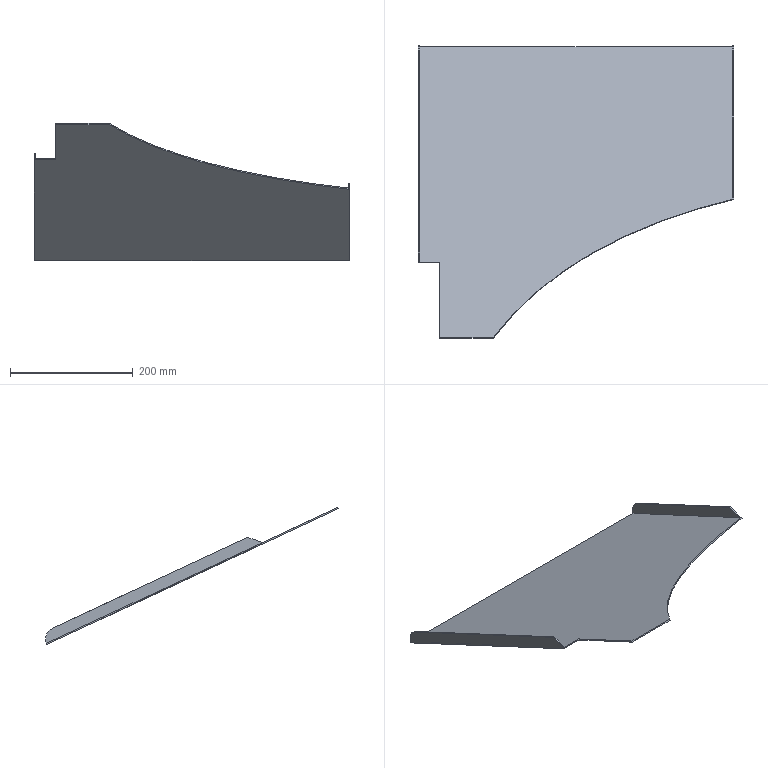Part | NX | features solid 2 | 1 solid | 17 faces | box 515 x 478.276 x 223.963 mm | volume 430449 mm3 | plane 14 | cylinder 2 | spline 1 | commonest cylinder face diameters 40 x2
STEP:
#1=CARTESIAN_POINT('',(-287.,720.,-282.15));
#2=VERTEX_POINT('',#1);
#3=CARTESIAN_POINT('',(-287.,720.,-279.943));
#4=VERTEX_POINT('',#3);
#5=CARTESIAN_POINT('',(-287.,720.,-430.));
#6=DIRECTION('',(0.,0.,1.));
#7=VECTOR('',#6,1000.);
#8=LINE('',#5,#7);
#9=EDGE_CURVE('',#2,#4,#8,.T.);
#10=ORIENTED_EDGE('',*,*,#9,.F.);
#11=CARTESIAN_POINT('',(-798.,720.,-282.15));
#12=VERTEX_POINT('',#11);
#13=CARTESIAN_POINT('',(188.564,720.,-282.15));
#14=DIRECTION('',(-1.,0.,0.));
#15=VECTOR('',#14,1000.);
#16=LINE('',#13,#15);
#17=EDGE_CURVE('',#2,#12,#16,.T.);
#18=ORIENTED_EDGE('',*,*,#17,.T.);
#19=CARTESIAN_POINT('',(-798.,720.,-279.943));
#20=VERTEX_POINT('',#19);
#21=CARTESIAN_POINT('',(-798.,720.,-430.));
#22=DIRECTION('',(0.,0.,-1.));
#23=VECTOR('',#22,1000.);
#24=LINE('',#21,#23);
#25=EDGE_CURVE('',#20,#12,#24,.T.);
#26=ORIENTED_EDGE('',*,*,#25,.F.);
#27=CARTESIAN_POINT('',(188.564,720.,-279.943));
#28=DIRECTION('',(-1.,0.,0.));
#29=VECTOR('',#28,1000.);
#30=LINE('',#27,#29);
#31=EDGE_CURVE('',#4,#20,#30,.T.);
#32=ORIENTED_EDGE('',*,*,#31,.F.);
#33=EDGE_LOOP('',(#10,#18,#26,#32));
#34=FACE_BOUND('',#33,.T.);
#35=CARTESIAN_POINT('',(188.564,720.,-430.));
#36=DIRECTION('',(0.,-1.,0.));
#37=DIRECTION('',(-1.,0.,0.));
#38=AXIS2_PLACEMENT_3D('',#35,#36,#37);
#39=PLANE('',#38);
#40=ADVANCED_FACE('',(#34),#39,.F.);
#41=CARTESIAN_POINT('',(-287.,472.974,-164.753));
#42=VERTEX_POINT('',#41);
#43=CARTESIAN_POINT('',(-285.,472.974,-164.753));
#44=VERTEX_POINT('',#43);
#45=CARTESIAN_POINT('',(-353.018,472.974,-164.753));
#46=DIRECTION('',(-1.,0.,0.));
#47=VECTOR('',#46,1000.);
#48=LINE('',#45,#47);
#49=EDGE_CURVE('',#42,#44,#48,.F.);
#50=ORIENTED_EDGE('',*,*,#49,.F.);
#51=CARTESIAN_POINT('',(-287.,417.055,-138.678));
#52=DIRECTION('',(0.,0.9063,-0.4226));
#53=VECTOR('',#52,1000.);
#54=LINE('',#51,#53);
#55=EDGE_CURVE('',#42,#4,#54,.T.);
#56=ORIENTED_EDGE('',*,*,#55,.T.);
#57=ORIENTED_EDGE('',*,*,#31,.T.);
#58=CARTESIAN_POINT('',(-798.,367.658,-115.644));
#59=VERTEX_POINT('',#58);
#60=CARTESIAN_POINT('',(-798.,417.055,-138.678));
#61=DIRECTION('',(0.,-0.9063,0.4226));
#62=VECTOR('',#61,1000.);
#63=LINE('',#60,#62);
#64=EDGE_CURVE('',#20,#59,#63,.T.);
#65=ORIENTED_EDGE('',*,*,#64,.T.);
#66=CARTESIAN_POINT('',(-765.,367.658,-115.644));
#67=VERTEX_POINT('',#66);
#68=CARTESIAN_POINT('',(-779.,367.658,-115.644));
#69=DIRECTION('',(-1.,0.,0.));
#70=VECTOR('',#69,1000.);
#71=LINE('',#68,#70);
#72=EDGE_CURVE('',#67,#59,#71,.T.);
#73=ORIENTED_EDGE('',*,*,#72,.F.);
#74=CARTESIAN_POINT('',(-765.,244.443,-58.187));
#75=VERTEX_POINT('',#74);
#76=CARTESIAN_POINT('',(-765.,272.567,-71.302));
#77=DIRECTION('',(0.,-0.9063,0.4226));
#78=VECTOR('',#77,1000.);
#79=LINE('',#76,#78);
#80=EDGE_CURVE('',#75,#67,#79,.F.);
#81=ORIENTED_EDGE('',*,*,#80,.F.);
#82=CARTESIAN_POINT('',(-677.72,244.443,-58.187));
#83=VERTEX_POINT('',#82);
#84=CARTESIAN_POINT('',(-353.018,244.443,-58.187));
#85=DIRECTION('',(1.,0.,0.));
#86=VECTOR('',#85,1000.);
#87=LINE('',#84,#86);
#88=EDGE_CURVE('',#75,#83,#87,.T.);
#89=ORIENTED_EDGE('',*,*,#88,.T.);
#90=CARTESIAN_POINT('',(-285.,471.162,-163.908));
#91=VERTEX_POINT('',#90);
#92=CARTESIAN_POINT('',(-677.72,244.443,-58.187));
#93=CARTESIAN_POINT('',(-672.167,251.77,-61.604));
#94=CARTESIAN_POINT('',(-663.423,262.605,-66.657));
#95=CARTESIAN_POINT('',(-650.978,276.698,-73.228));
#96=CARTESIAN_POINT('',(-641.165,287.179,-78.116));
#97=CARTESIAN_POINT('',(-631.216,297.219,-82.798));
#98=CARTESIAN_POINT('',(-620.962,307.004,-87.36));
#99=CARTESIAN_POINT('',(-612.158,314.946,-91.063));
#100=CARTESIAN_POINT('',(-604.955,321.177,-93.969));
#101=CARTESIAN_POINT('',(-600.401,325.008,-95.756));
#102=CARTESIAN_POINT('',(-596.688,328.067,-97.182));
#103=CARTESIAN_POINT('',(-593.065,331.011,-98.555));
#104=CARTESIAN_POINT('',(-586.789,336.01,-100.886));
#105=CARTESIAN_POINT('',(-573.857,345.914,-105.504));
#106=CARTESIAN_POINT('',(-558.47,356.808,-110.584));
#107=CARTESIAN_POINT('',(-542.419,367.323,-115.487));
#108=CARTESIAN_POINT('',(-530.057,375.012,-119.073));
#109=CARTESIAN_POINT('',(-517.377,382.503,-122.566));
#110=CARTESIAN_POINT('',(-506.516,388.595,-125.406));
#111=CARTESIAN_POINT('',(-498.82,392.748,-127.343));
#112=CARTESIAN_POINT('',(-494.304,395.136,-128.457));
#113=CARTESIAN_POINT('',(-490.241,397.26,-129.447));
#114=CARTESIAN_POINT('',(-484.961,399.97,-130.711));
#115=CARTESIAN_POINT('',(-476.523,404.197,-132.682));
#116=CARTESIAN_POINT('',(-465.791,409.379,-135.099));
#117=CARTESIAN_POINT('',(-448.313,417.413,-138.845));
#118=CARTESIAN_POINT('',(-430.339,425.076,-142.418));
#119=CARTESIAN_POINT('',(-411.886,432.361,-145.815));
#120=CARTESIAN_POINT('',(-400.134,436.764,-147.868));
#121=CARTESIAN_POINT('',(-390.645,440.181,-149.462));
#122=CARTESIAN_POINT('',(-383.373,442.729,-150.65));
#123=CARTESIAN_POINT('',(-376.401,445.108,-151.759));
#124=CARTESIAN_POINT('',(-367.079,448.209,-153.205));
#125=CARTESIAN_POINT('',(-357.741,451.192,-154.596));
#126=CARTESIAN_POINT('',(-348.382,454.06,-155.933));
#127=CARTESIAN_POINT('',(-341.353,456.153,-156.91));
#128=CARTESIAN_POINT('',(-335.488,457.849,-157.7));
#129=CARTESIAN_POINT('',(-330.79,459.178,-158.32));
#130=CARTESIAN_POINT('',(-327.855,459.995,-158.701));
#131=CARTESIAN_POINT('',(-325.793,460.562,-158.966));
#132=CARTESIAN_POINT('',(-324.625,460.882,-159.115));
#133=CARTESIAN_POINT('',(-323.869,461.088,-159.211));
#134=CARTESIAN_POINT('',(-323.323,461.236,-159.28));
#135=CARTESIAN_POINT('',(-322.949,461.338,-159.327));
#136=CARTESIAN_POINT('',(-322.199,461.541,-159.422));
#137=CARTESIAN_POINT('',(-320.706,461.943,-159.609));
#138=CARTESIAN_POINT('',(-318.393,462.561,-159.898));
#139=CARTESIAN_POINT('',(-314.394,463.619,-160.391));
#140=CARTESIAN_POINT('',(-308.795,465.082,-161.073));
#141=CARTESIAN_POINT('',(-302.405,466.73,-161.842));
#142=CARTESIAN_POINT('',(-297.517,467.981,-162.425));
#143=CARTESIAN_POINT('',(-294.603,468.725,-162.772));
#144=CARTESIAN_POINT('',(-292.74,469.199,-162.993));
#145=CARTESIAN_POINT('',(-291.2,469.59,-163.175));
#146=CARTESIAN_POINT('',(-290.27,469.826,-163.286));
#147=CARTESIAN_POINT('',(-289.417,470.043,-163.386));
#148=CARTESIAN_POINT('',(-288.93,470.166,-163.444));
#149=CARTESIAN_POINT('',(-287.978,470.408,-163.557));
#150=CARTESIAN_POINT('',(-286.649,470.744,-163.714));
#151=CARTESIAN_POINT('',(-285.552,471.022,-163.843));
#152=CARTESIAN_POINT('',(-285.,471.162,-163.908));
#153=B_SPLINE_CURVE_WITH_KNOTS('',3,(#92,#93,#94,#95,#96,#97,#98,#99,#100,#101,#102,#103,#104,#105,#106,#107,#108,#109,#110,#111,#112,#113,#114,#115,#116,#117,#118,#119,#120,#121,#122,#123,#124,#125,#126,#127,#128,#129,#130,#131,#132,#133,#134,#135,#136,#137,#138,#139,#140,#141,#142,#143,#144,#145,#146,#147,#148,#149,#150,#151,#152),.UNSPECIFIED.,.F.,.F.,(4,1,1,1,1,1,1,1,1,1,1,1,1,1,1,1,1,1,1,1,1,1,1,1,1,1,1,1,1,1,1,1,1,1,1,1,1,1,1,1,1,1,1,1,1,1,1,1,1,1,1,1,1,1,1,1,1,1,4),(0.,0.02989,0.04484,0.05979,0.07473,0.08968,0.1046,0.1121,0.1196,0.1233,0.127,0.1345,0.1495,0.1794,0.1943,0.2093,0.2242,0.2392,0.2466,0.2504,0.2541,0.2616,0.269,0.284,0.2989,0.3288,0.3438,0.3587,0.3662,0.3737,0.3811,0.3886,0.4036,0.411,0.4185,0.426,0.4297,0.4335,0.4353,0.4363,0.4372,0.4377,0.4381,0.4391,0.4409,0.4447,0.4484,0.4559,0.4634,0.4671,0.469,0.4708,0.4718,0.4727,0.4732,0.4736,0.4746,0.4764,0.4783),.UNSPECIFIED.);
#154=EDGE_CURVE('',#83,#91,#153,.T.);
#155=ORIENTED_EDGE('',*,*,#154,.T.);
#156=CARTESIAN_POINT('',(-285.,417.055,-138.678));
#157=DIRECTION('',(0.,0.9063,-0.4226));
#158=VECTOR('',#157,1000.);
#159=LINE('',#156,#158);
#160=EDGE_CURVE('',#91,#44,#159,.T.);
#161=ORIENTED_EDGE('',*,*,#160,.T.);
#162=EDGE_LOOP('',(#50,#56,#57,#65,#73,#81,#89,#155,#161));
#163=FACE_BOUND('',#162,.T.);
#164=CARTESIAN_POINT('',(-353.018,417.055,-138.678));
#165=DIRECTION('',(0.,0.4226,0.9063));
#166=DIRECTION('',(1.,0.,0.));
#167=AXIS2_PLACEMENT_3D('',#164,#165,#166);
#168=PLANE('',#167);
#169=ADVANCED_FACE('',(#163),#168,.T.);
#170=CARTESIAN_POINT('',(-285.,470.316,-165.721));
#171=VERTEX_POINT('',#170);
#172=CARTESIAN_POINT('',(-285.,471.162,-163.908));
#173=DIRECTION('',(0.,-0.4226,-0.9063));
#174=VECTOR('',#173,1000.);
#175=LINE('',#172,#174);
#176=EDGE_CURVE('',#91,#171,#175,.T.);
#177=ORIENTED_EDGE('',*,*,#176,.F.);
#178=ORIENTED_EDGE('',*,*,#154,.F.);
#179=CARTESIAN_POINT('',(-677.72,243.597,-60.));
#180=VERTEX_POINT('',#179);
#181=CARTESIAN_POINT('',(-677.72,243.597,-60.));
#182=CARTESIAN_POINT('',(-677.72,243.879,-59.396));
#183=CARTESIAN_POINT('',(-677.72,244.161,-58.792));
#184=CARTESIAN_POINT('',(-677.72,244.443,-58.187));
#185=B_SPLINE_CURVE_WITH_KNOTS('',3,(#181,#182,#183,#184),.UNSPECIFIED.,.F.,.F.,(4,4),(0.,1.),.UNSPECIFIED.);
#186=EDGE_CURVE('',#83,#180,#185,.F.);
#187=ORIENTED_EDGE('',*,*,#186,.T.);
#188=CARTESIAN_POINT('',(-677.72,243.597,-60.));
#189=CARTESIAN_POINT('',(-672.167,250.924,-63.417));
#190=CARTESIAN_POINT('',(-663.423,261.76,-68.469));
#191=CARTESIAN_POINT('',(-650.978,275.853,-75.041));
#192=CARTESIAN_POINT('',(-641.165,286.334,-79.928));
#193=CARTESIAN_POINT('',(-631.216,296.374,-84.61));
#194=CARTESIAN_POINT('',(-620.962,306.159,-89.173));
#195=CARTESIAN_POINT('',(-612.158,314.1,-92.876));
#196=CARTESIAN_POINT('',(-604.955,320.332,-95.782));
#197=CARTESIAN_POINT('',(-600.401,324.163,-97.568));
#198=CARTESIAN_POINT('',(-596.688,327.222,-98.995));
#199=CARTESIAN_POINT('',(-593.065,330.165,-100.367));
#200=CARTESIAN_POINT('',(-586.789,335.164,-102.698));
#201=CARTESIAN_POINT('',(-573.857,345.068,-107.317));
#202=CARTESIAN_POINT('',(-558.47,355.963,-112.397));
#203=CARTESIAN_POINT('',(-542.419,366.477,-117.3));
#204=CARTESIAN_POINT('',(-530.057,374.167,-120.886));
#205=CARTESIAN_POINT('',(-517.377,381.657,-124.378));
#206=CARTESIAN_POINT('',(-506.516,387.749,-127.219));
#207=CARTESIAN_POINT('',(-498.82,391.902,-129.156));
#208=CARTESIAN_POINT('',(-494.304,394.291,-130.27));
#209=CARTESIAN_POINT('',(-490.241,396.414,-131.26));
#210=CARTESIAN_POINT('',(-484.961,399.125,-132.524));
#211=CARTESIAN_POINT('',(-476.523,403.351,-134.494));
#212=CARTESIAN_POINT('',(-465.791,408.534,-136.911));
#213=CARTESIAN_POINT('',(-448.313,416.568,-140.657));
#214=CARTESIAN_POINT('',(-430.339,424.231,-144.231));
#215=CARTESIAN_POINT('',(-411.886,431.516,-147.628));
#216=CARTESIAN_POINT('',(-400.134,435.919,-149.681));
#217=CARTESIAN_POINT('',(-390.645,439.336,-151.274));
#218=CARTESIAN_POINT('',(-383.373,441.884,-152.463));
#219=CARTESIAN_POINT('',(-376.401,444.263,-153.572));
#220=CARTESIAN_POINT('',(-367.079,447.363,-155.018));
#221=CARTESIAN_POINT('',(-357.741,450.347,-156.409));
#222=CARTESIAN_POINT('',(-348.382,453.215,-157.746));
#223=CARTESIAN_POINT('',(-341.353,455.308,-158.722));
#224=CARTESIAN_POINT('',(-335.488,457.004,-159.513));
#225=CARTESIAN_POINT('',(-330.79,458.332,-160.133));
#226=CARTESIAN_POINT('',(-327.855,459.15,-160.514));
#227=CARTESIAN_POINT('',(-325.793,459.717,-160.778));
#228=CARTESIAN_POINT('',(-324.625,460.037,-160.927));
#229=CARTESIAN_POINT('',(-323.869,460.243,-161.023));
#230=CARTESIAN_POINT('',(-323.323,460.391,-161.093));
#231=CARTESIAN_POINT('',(-322.949,460.493,-161.14));
#232=CARTESIAN_POINT('',(-322.199,460.696,-161.235));
#233=CARTESIAN_POINT('',(-320.706,461.098,-161.422));
#234=CARTESIAN_POINT('',(-318.393,461.716,-161.71));
#235=CARTESIAN_POINT('',(-314.394,462.773,-162.203));
#236=CARTESIAN_POINT('',(-308.795,464.237,-162.886));
#237=CARTESIAN_POINT('',(-302.405,465.885,-163.654));
#238=CARTESIAN_POINT('',(-297.517,467.136,-164.238));
#239=CARTESIAN_POINT('',(-294.603,467.88,-164.584));
#240=CARTESIAN_POINT('',(-292.74,468.354,-164.806));
#241=CARTESIAN_POINT('',(-291.2,468.745,-164.988));
#242=CARTESIAN_POINT('',(-290.27,468.981,-165.098));
#243=CARTESIAN_POINT('',(-289.417,469.198,-165.199));
#244=CARTESIAN_POINT('',(-288.93,469.321,-165.257));
#245=CARTESIAN_POINT('',(-287.978,469.562,-165.369));
#246=CARTESIAN_POINT('',(-286.649,469.899,-165.526));
#247=CARTESIAN_POINT('',(-285.552,470.177,-165.656));
#248=CARTESIAN_POINT('',(-285.,470.316,-165.721));
#249=B_SPLINE_CURVE_WITH_KNOTS('',3,(#188,#189,#190,#191,#192,#193,#194,#195,#196,#197,#198,#199,#200,#201,#202,#203,#204,#205,#206,#207,#208,#209,#210,#211,#212,#213,#214,#215,#216,#217,#218,#219,#220,#221,#222,#223,#224,#225,#226,#227,#228,#229,#230,#231,#232,#233,#234,#235,#236,#237,#238,#239,#240,#241,#242,#243,#244,#245,#246,#247,#248),.UNSPECIFIED.,.F.,.F.,(4,1,1,1,1,1,1,1,1,1,1,1,1,1,1,1,1,1,1,1,1,1,1,1,1,1,1,1,1,1,1,1,1,1,1,1,1,1,1,1,1,1,1,1,1,1,1,1,1,1,1,1,1,1,1,1,1,1,4),(0.,0.02989,0.04484,0.05979,0.07473,0.08968,0.1046,0.1121,0.1196,0.1233,0.127,0.1345,0.1495,0.1794,0.1943,0.2093,0.2242,0.2392,0.2466,0.2504,0.2541,0.2616,0.269,0.284,0.2989,0.3288,0.3438,0.3587,0.3662,0.3737,0.3811,0.3886,0.4036,0.411,0.4185,0.426,0.4297,0.4335,0.4353,0.4363,0.4372,0.4377,0.4381,0.4391,0.4409,0.4447,0.4484,0.4559,0.4634,0.4671,0.469,0.4708,0.4718,0.4727,0.4732,0.4736,0.4746,0.4764,0.4783),.UNSPECIFIED.);
#250=EDGE_CURVE('',#180,#171,#249,.T.);
#251=ORIENTED_EDGE('',*,*,#250,.T.);
#252=EDGE_LOOP('',(#177,#178,#187,#251));
#253=FACE_BOUND('',#252,.T.);
#254=CARTESIAN_POINT('',(-677.72,244.443,-58.187));
#255=CARTESIAN_POINT('',(-677.72,243.597,-60.));
#256=CARTESIAN_POINT('',(-672.167,251.77,-61.604));
#257=CARTESIAN_POINT('',(-672.167,250.924,-63.417));
#258=CARTESIAN_POINT('',(-663.423,262.605,-66.657));
#259=CARTESIAN_POINT('',(-663.423,261.76,-68.469));
#260=CARTESIAN_POINT('',(-650.978,276.698,-73.228));
#261=CARTESIAN_POINT('',(-650.978,275.853,-75.041));
#262=CARTESIAN_POINT('',(-641.165,287.179,-78.116));
#263=CARTESIAN_POINT('',(-641.165,286.334,-79.928));
#264=CARTESIAN_POINT('',(-631.216,297.219,-82.798));
#265=CARTESIAN_POINT('',(-631.216,296.374,-84.61));
#266=CARTESIAN_POINT('',(-620.962,307.004,-87.36));
#267=CARTESIAN_POINT('',(-620.962,306.159,-89.173));
#268=CARTESIAN_POINT('',(-612.158,314.946,-91.063));
#269=CARTESIAN_POINT('',(-612.158,314.1,-92.876));
#270=CARTESIAN_POINT('',(-604.955,321.177,-93.969));
#271=CARTESIAN_POINT('',(-604.955,320.332,-95.782));
#272=CARTESIAN_POINT('',(-600.401,325.008,-95.756));
#273=CARTESIAN_POINT('',(-600.401,324.163,-97.568));
#274=CARTESIAN_POINT('',(-596.688,328.067,-97.182));
#275=CARTESIAN_POINT('',(-596.688,327.222,-98.995));
#276=CARTESIAN_POINT('',(-593.065,331.011,-98.555));
#277=CARTESIAN_POINT('',(-593.065,330.165,-100.367));
#278=CARTESIAN_POINT('',(-586.789,336.01,-100.886));
#279=CARTESIAN_POINT('',(-586.789,335.164,-102.698));
#280=CARTESIAN_POINT('',(-573.857,345.914,-105.504));
#281=CARTESIAN_POINT('',(-573.857,345.068,-107.317));
#282=CARTESIAN_POINT('',(-558.47,356.808,-110.584));
#283=CARTESIAN_POINT('',(-558.47,355.963,-112.397));
#284=CARTESIAN_POINT('',(-542.419,367.323,-115.487));
#285=CARTESIAN_POINT('',(-542.419,366.477,-117.3));
#286=CARTESIAN_POINT('',(-530.057,375.012,-119.073));
#287=CARTESIAN_POINT('',(-530.057,374.167,-120.886));
#288=CARTESIAN_POINT('',(-517.377,382.503,-122.566));
#289=CARTESIAN_POINT('',(-517.377,381.657,-124.378));
#290=CARTESIAN_POINT('',(-506.516,388.595,-125.406));
#291=CARTESIAN_POINT('',(-506.516,387.749,-127.219));
#292=CARTESIAN_POINT('',(-498.82,392.748,-127.343));
#293=CARTESIAN_POINT('',(-498.82,391.902,-129.156));
#294=CARTESIAN_POINT('',(-494.304,395.136,-128.457));
#295=CARTESIAN_POINT('',(-494.304,394.291,-130.27));
#296=CARTESIAN_POINT('',(-490.241,397.26,-129.447));
#297=CARTESIAN_POINT('',(-490.241,396.414,-131.26));
#298=CARTESIAN_POINT('',(-484.961,399.97,-130.711));
#299=CARTESIAN_POINT('',(-484.961,399.125,-132.524));
#300=CARTESIAN_POINT('',(-476.523,404.197,-132.682));
#301=CARTESIAN_POINT('',(-476.523,403.351,-134.494));
#302=CARTESIAN_POINT('',(-465.791,409.379,-135.099));
#303=CARTESIAN_POINT('',(-465.791,408.534,-136.911));
#304=CARTESIAN_POINT('',(-448.313,417.413,-138.845));
#305=CARTESIAN_POINT('',(-448.313,416.568,-140.657));
#306=CARTESIAN_POINT('',(-430.339,425.076,-142.418));
#307=CARTESIAN_POINT('',(-430.339,424.231,-144.231));
#308=CARTESIAN_POINT('',(-411.886,432.361,-145.815));
#309=CARTESIAN_POINT('',(-411.886,431.516,-147.628));
#310=CARTESIAN_POINT('',(-400.134,436.764,-147.868));
#311=CARTESIAN_POINT('',(-400.134,435.919,-149.681));
#312=CARTESIAN_POINT('',(-390.645,440.181,-149.462));
#313=CARTESIAN_POINT('',(-390.645,439.336,-151.274));
#314=CARTESIAN_POINT('',(-383.373,442.729,-150.65));
#315=CARTESIAN_POINT('',(-383.373,441.884,-152.463));
#316=CARTESIAN_POINT('',(-376.401,445.108,-151.759));
#317=CARTESIAN_POINT('',(-376.401,444.263,-153.572));
#318=CARTESIAN_POINT('',(-367.079,448.209,-153.205));
#319=CARTESIAN_POINT('',(-367.079,447.363,-155.018));
#320=CARTESIAN_POINT('',(-357.741,451.192,-154.596));
#321=CARTESIAN_POINT('',(-357.741,450.347,-156.409));
#322=CARTESIAN_POINT('',(-348.382,454.06,-155.933));
#323=CARTESIAN_POINT('',(-348.382,453.215,-157.746));
#324=CARTESIAN_POINT('',(-341.353,456.153,-156.91));
#325=CARTESIAN_POINT('',(-341.353,455.308,-158.722));
#326=CARTESIAN_POINT('',(-335.488,457.849,-157.7));
#327=CARTESIAN_POINT('',(-335.488,457.004,-159.513));
#328=CARTESIAN_POINT('',(-330.79,459.178,-158.32));
#329=CARTESIAN_POINT('',(-330.79,458.332,-160.133));
#330=CARTESIAN_POINT('',(-327.855,459.995,-158.701));
#331=CARTESIAN_POINT('',(-327.855,459.15,-160.514));
#332=CARTESIAN_POINT('',(-325.793,460.562,-158.966));
#333=CARTESIAN_POINT('',(-325.793,459.717,-160.778));
#334=CARTESIAN_POINT('',(-324.625,460.882,-159.115));
#335=CARTESIAN_POINT('',(-324.625,460.037,-160.927));
#336=CARTESIAN_POINT('',(-323.869,461.088,-159.211));
#337=CARTESIAN_POINT('',(-323.869,460.243,-161.023));
#338=CARTESIAN_POINT('',(-323.323,461.236,-159.28));
#339=CARTESIAN_POINT('',(-323.323,460.391,-161.093));
#340=CARTESIAN_POINT('',(-322.949,461.338,-159.327));
#341=CARTESIAN_POINT('',(-322.949,460.493,-161.14));
#342=CARTESIAN_POINT('',(-322.199,461.541,-159.422));
#343=CARTESIAN_POINT('',(-322.199,460.696,-161.235));
#344=CARTESIAN_POINT('',(-320.706,461.943,-159.609));
#345=CARTESIAN_POINT('',(-320.706,461.098,-161.422));
#346=CARTESIAN_POINT('',(-318.393,462.561,-159.898));
#347=CARTESIAN_POINT('',(-318.393,461.716,-161.71));
#348=CARTESIAN_POINT('',(-314.394,463.619,-160.391));
#349=CARTESIAN_POINT('',(-314.394,462.773,-162.203));
#350=CARTESIAN_POINT('',(-308.795,465.082,-161.073));
#351=CARTESIAN_POINT('',(-308.795,464.237,-162.886));
#352=CARTESIAN_POINT('',(-302.405,466.73,-161.842));
#353=CARTESIAN_POINT('',(-302.405,465.885,-163.654));
#354=CARTESIAN_POINT('',(-297.517,467.981,-162.425));
#355=CARTESIAN_POINT('',(-297.517,467.136,-164.238));
#356=CARTESIAN_POINT('',(-294.603,468.725,-162.772));
#357=CARTESIAN_POINT('',(-294.603,467.88,-164.584));
#358=CARTESIAN_POINT('',(-292.74,469.199,-162.993));
#359=CARTESIAN_POINT('',(-292.74,468.354,-164.806));
#360=CARTESIAN_POINT('',(-291.2,469.59,-163.175));
#361=CARTESIAN_POINT('',(-291.2,468.745,-164.988));
#362=CARTESIAN_POINT('',(-290.27,469.826,-163.286));
#363=CARTESIAN_POINT('',(-290.27,468.981,-165.098));
#364=CARTESIAN_POINT('',(-289.417,470.043,-163.386));
#365=CARTESIAN_POINT('',(-289.417,469.198,-165.199));
#366=CARTESIAN_POINT('',(-288.93,470.166,-163.444));
#367=CARTESIAN_POINT('',(-288.93,469.321,-165.257));
#368=CARTESIAN_POINT('',(-287.978,470.408,-163.557));
#369=CARTESIAN_POINT('',(-287.978,469.562,-165.369));
#370=CARTESIAN_POINT('',(-286.649,470.744,-163.714));
#371=CARTESIAN_POINT('',(-286.649,469.899,-165.526));
#372=CARTESIAN_POINT('',(-285.552,471.022,-163.843));
#373=CARTESIAN_POINT('',(-285.552,470.177,-165.656));
#374=CARTESIAN_POINT('',(-285.,471.162,-163.908));
#375=CARTESIAN_POINT('',(-285.,470.316,-165.721));
#376=B_SPLINE_SURFACE_WITH_KNOTS('',3,1,((#254,#255),(#256,#257),(#258,#259),(#260,#261),(#262,#263),(#264,#265),(#266,#267),(#268,#269),(#270,#271),(#272,#273),(#274,#275),(#276,#277),(#278,#279),(#280,#281),(#282,#283),(#284,#285),(#286,#287),(#288,#289),(#290,#291),(#292,#293),(#294,#295),(#296,#297),(#298,#299),(#300,#301),(#302,#303),(#304,#305),(#306,#307),(#308,#309),(#310,#311),(#312,#313),(#314,#315),(#316,#317),(#318,#319),(#320,#321),(#322,#323),(#324,#325),(#326,#327),(#328,#329),(#330,#331),(#332,#333),(#334,#335),(#336,#337),(#338,#339),(#340,#341),(#342,#343),(#344,#345),(#346,#347),(#348,#349),(#350,#351),(#352,#353),(#354,#355),(#356,#357),(#358,#359),(#360,#361),(#362,#363),(#364,#365),(#366,#367),(#368,#369),(#370,#371),(#372,#373),(#374,#375)),.SURF_OF_LINEAR_EXTRUSION.,.F.,.F.,.F.,(4,1,1,1,1,1,1,1,1,1,1,1,1,1,1,1,1,1,1,1,1,1,1,1,1,1,1,1,1,1,1,1,1,1,1,1,1,1,1,1,1,1,1,1,1,1,1,1,1,1,1,1,1,1,1,1,1,1,4),(2,2),(0.,0.02989,0.04484,0.05979,0.07473,0.08968,0.1046,0.1121,0.1196,0.1233,0.127,0.1345,0.1495,0.1794,0.1943,0.2093,0.2242,0.2392,0.2466,0.2504,0.2541,0.2616,0.269,0.284,0.2989,0.3288,0.3438,0.3587,0.3662,0.3737,0.3811,0.3886,0.4036,0.411,0.4185,0.426,0.4297,0.4335,0.4353,0.4363,0.4372,0.4377,0.4381,0.4391,0.4409,0.4447,0.4484,0.4559,0.4634,0.4671,0.469,0.4708,0.4718,0.4727,0.4732,0.4736,0.4746,0.4764,0.4783),(0.,1.),.UNSPECIFIED.);
#377=ADVANCED_FACE('',(#253),#376,.F.);
#378=ORIENTED_EDGE('',*,*,#17,.F.);
#379=CARTESIAN_POINT('',(-285.,720.,-282.15));
#380=VERTEX_POINT('',#379);
#381=CARTESIAN_POINT('',(188.564,720.,-282.15));
#382=DIRECTION('',(-1.,0.,0.));
#383=VECTOR('',#382,1000.);
#384=LINE('',#381,#383);
#385=EDGE_CURVE('',#380,#2,#384,.T.);
#386=ORIENTED_EDGE('',*,*,#385,.F.);
#387=CARTESIAN_POINT('',(-285.,416.21,-140.491));
#388=DIRECTION('',(0.,0.9063,-0.4226));
#389=VECTOR('',#388,1000.);
#390=LINE('',#387,#389);
#391=EDGE_CURVE('',#171,#380,#390,.T.);
#392=ORIENTED_EDGE('',*,*,#391,.F.);
#393=ORIENTED_EDGE('',*,*,#250,.F.);
#394=CARTESIAN_POINT('',(-765.,243.597,-60.));
#395=VERTEX_POINT('',#394);
#396=CARTESIAN_POINT('',(-353.018,243.597,-60.));
#397=DIRECTION('',(1.,0.,0.));
#398=VECTOR('',#397,1000.);
#399=LINE('',#396,#398);
#400=EDGE_CURVE('',#395,#180,#399,.T.);
#401=ORIENTED_EDGE('',*,*,#400,.F.);
#402=CARTESIAN_POINT('',(-765.,366.813,-117.456));
#403=VERTEX_POINT('',#402);
#404=CARTESIAN_POINT('',(-765.,271.722,-73.114));
#405=DIRECTION('',(0.,-0.9063,0.4226));
#406=VECTOR('',#405,1000.);
#407=LINE('',#404,#406);
#408=EDGE_CURVE('',#395,#403,#407,.F.);
#409=ORIENTED_EDGE('',*,*,#408,.T.);
#410=CARTESIAN_POINT('',(-800.,366.813,-117.456));
#411=VERTEX_POINT('',#410);
#412=CARTESIAN_POINT('',(-779.,366.813,-117.456));
#413=DIRECTION('',(-1.,0.,0.));
#414=VECTOR('',#413,1000.);
#415=LINE('',#412,#414);
#416=EDGE_CURVE('',#403,#411,#415,.T.);
#417=ORIENTED_EDGE('',*,*,#416,.T.);
#418=CARTESIAN_POINT('',(-800.,720.,-282.15));
#419=VERTEX_POINT('',#418);
#420=CARTESIAN_POINT('',(-800.,559.597,-207.353));
#421=DIRECTION('',(0.,-0.9063,0.4226));
#422=VECTOR('',#421,1000.);
#423=LINE('',#420,#422);
#424=EDGE_CURVE('',#419,#411,#423,.T.);
#425=ORIENTED_EDGE('',*,*,#424,.F.);
#426=CARTESIAN_POINT('',(-800.,720.,-282.15));
#427=DIRECTION('',(1.,0.,0.));
#428=VECTOR('',#427,1000.);
#429=LINE('',#426,#428);
#430=EDGE_CURVE('',#419,#12,#429,.T.);
#431=ORIENTED_EDGE('',*,*,#430,.T.);
#432=EDGE_LOOP('',(#378,#386,#392,#393,#401,#409,#417,#425,#431));
#433=FACE_BOUND('',#432,.T.);
#434=CARTESIAN_POINT('',(-353.018,416.21,-140.491));
#435=DIRECTION('',(0.,0.4226,0.9063));
#436=DIRECTION('',(1.,0.,0.));
#437=AXIS2_PLACEMENT_3D('',#434,#435,#436);
#438=PLANE('',#437);
#439=ADVANCED_FACE('',(#433),#438,.F.);
#440=ORIENTED_EDGE('',*,*,#72,.T.);
#441=CARTESIAN_POINT('',(-800.,367.658,-115.644));
#442=VERTEX_POINT('',#441);
#443=CARTESIAN_POINT('',(-779.,367.658,-115.644));
#444=DIRECTION('',(-1.,0.,0.));
#445=VECTOR('',#444,1000.);
#446=LINE('',#443,#445);
#447=EDGE_CURVE('',#59,#442,#446,.T.);
#448=ORIENTED_EDGE('',*,*,#447,.T.);
#449=CARTESIAN_POINT('',(-800.,367.658,-115.644));
#450=DIRECTION('',(0.,-0.4226,-0.9063));
#451=VECTOR('',#450,1000.);
#452=LINE('',#449,#451);
#453=EDGE_CURVE('',#442,#411,#452,.T.);
#454=ORIENTED_EDGE('',*,*,#453,.T.);
#455=ORIENTED_EDGE('',*,*,#416,.F.);
#456=CARTESIAN_POINT('',(-765.,367.658,-115.644));
#457=DIRECTION('',(0.,-0.4226,-0.9063));
#458=VECTOR('',#457,1000.);
#459=LINE('',#456,#458);
#460=EDGE_CURVE('',#67,#403,#459,.T.);
#461=ORIENTED_EDGE('',*,*,#460,.F.);
#462=EDGE_LOOP('',(#440,#448,#454,#455,#461));
#463=FACE_BOUND('',#462,.T.);
#464=CARTESIAN_POINT('',(-779.,367.658,-115.644));
#465=DIRECTION('',(0.,-0.9063,0.4226));
#466=DIRECTION('',(0.,-0.4226,-0.9063));
#467=AXIS2_PLACEMENT_3D('',#464,#465,#466);
#468=PLANE('',#467);
#469=ADVANCED_FACE('',(#463),#468,.T.);
#470=ORIENTED_EDGE('',*,*,#408,.F.);
#471=CARTESIAN_POINT('',(-765.,244.443,-58.187));
#472=DIRECTION('',(0.,0.4226,0.9063));
#473=VECTOR('',#472,1000.);
#474=LINE('',#471,#473);
#475=EDGE_CURVE('',#395,#75,#474,.T.);
#476=ORIENTED_EDGE('',*,*,#475,.T.);
#477=ORIENTED_EDGE('',*,*,#80,.T.);
#478=ORIENTED_EDGE('',*,*,#460,.T.);
#479=EDGE_LOOP('',(#470,#476,#477,#478));
#480=FACE_BOUND('',#479,.T.);
#481=CARTESIAN_POINT('',(-765.,272.567,-71.302));
#482=DIRECTION('',(-1.,0.,0.));
#483=DIRECTION('',(0.,0.,1.));
#484=AXIS2_PLACEMENT_3D('',#481,#482,#483);
#485=PLANE('',#484);
#486=ADVANCED_FACE('',(#480),#485,.T.);
#487=ORIENTED_EDGE('',*,*,#475,.F.);
#488=ORIENTED_EDGE('',*,*,#400,.T.);
#489=ORIENTED_EDGE('',*,*,#186,.F.);
#490=ORIENTED_EDGE('',*,*,#88,.F.);
#491=EDGE_LOOP('',(#487,#488,#489,#490));
#492=FACE_BOUND('',#491,.T.);
#493=CARTESIAN_POINT('',(-353.018,244.443,-58.187));
#494=DIRECTION('',(0.,0.9063,-0.4226));
#495=DIRECTION('',(0.,0.4226,0.9063));
#496=AXIS2_PLACEMENT_3D('',#493,#494,#495);
#497=PLANE('',#496);
#498=ADVANCED_FACE('',(#492),#497,.F.);
#499=ORIENTED_EDGE('',*,*,#453,.F.);
#500=CARTESIAN_POINT('',(-800.,391.579,-106.937));
#501=VERTEX_POINT('',#500);
#502=CARTESIAN_POINT('',(-800.,367.658,-115.644));
#503=DIRECTION('',(0.,0.9397,0.342));
#504=VECTOR('',#503,1000.);
#505=LINE('',#502,#504);
#506=EDGE_CURVE('',#442,#501,#505,.T.);
#507=ORIENTED_EDGE('',*,*,#506,.T.);
#508=CARTESIAN_POINT('',(-800.,710.326,-255.572));
#509=VERTEX_POINT('',#508);
#510=CARTESIAN_POINT('',(-800.,728.452,-264.024));
#511=DIRECTION('',(0.,-0.9063,0.4226));
#512=VECTOR('',#511,1000.);
#513=LINE('',#510,#512);
#514=EDGE_CURVE('',#509,#501,#513,.T.);
#515=ORIENTED_EDGE('',*,*,#514,.F.);
#516=CARTESIAN_POINT('',(-800.,701.874,-273.698));
#517=DIRECTION('',(-1.,0.,0.));
#518=DIRECTION('',(0.,0.,1.));
#519=AXIS2_PLACEMENT_3D('',#516,#517,#518);
#520=CIRCLE('',#519,20.);
#521=EDGE_CURVE('',#509,#419,#520,.T.);
#522=ORIENTED_EDGE('',*,*,#521,.T.);
#523=ORIENTED_EDGE('',*,*,#424,.T.);
#524=EDGE_LOOP('',(#499,#507,#515,#522,#523));
#525=FACE_BOUND('',#524,.T.);
#526=CARTESIAN_POINT('',(-800.,560.442,-205.54));
#527=DIRECTION('',(1.,0.,0.));
#528=DIRECTION('',(0.,0.,-1.));
#529=AXIS2_PLACEMENT_3D('',#526,#527,#528);
#530=PLANE('',#529);
#531=ADVANCED_FACE('',(#525),#530,.F.);
#532=CARTESIAN_POINT('',(-798.,710.326,-255.572));
#533=VERTEX_POINT('',#532);
#534=CARTESIAN_POINT('',(-798.,391.579,-106.937));
#535=VERTEX_POINT('',#534);
#536=CARTESIAN_POINT('',(-798.,728.452,-264.024));
#537=DIRECTION('',(0.,-0.9063,0.4226));
#538=VECTOR('',#537,1000.);
#539=LINE('',#536,#538);
#540=EDGE_CURVE('',#533,#535,#539,.T.);
#541=ORIENTED_EDGE('',*,*,#540,.T.);
#542=CARTESIAN_POINT('',(-798.,367.658,-115.644));
#543=DIRECTION('',(0.,-0.9397,-0.342));
#544=VECTOR('',#543,1000.);
#545=LINE('',#542,#544);
#546=EDGE_CURVE('',#535,#59,#545,.T.);
#547=ORIENTED_EDGE('',*,*,#546,.T.);
#548=ORIENTED_EDGE('',*,*,#64,.F.);
#549=ORIENTED_EDGE('',*,*,#25,.T.);
#550=CARTESIAN_POINT('',(-798.,701.874,-273.698));
#551=DIRECTION('',(-1.,0.,0.));
#552=DIRECTION('',(0.,0.,1.));
#553=AXIS2_PLACEMENT_3D('',#550,#551,#552);
#554=CIRCLE('',#553,20.);
#555=EDGE_CURVE('',#12,#533,#554,.F.);
#556=ORIENTED_EDGE('',*,*,#555,.T.);
#557=EDGE_LOOP('',(#541,#547,#548,#549,#556));
#558=FACE_BOUND('',#557,.T.);
#559=CARTESIAN_POINT('',(-798.,720.,-282.15));
#560=DIRECTION('',(-1.,0.,0.));
#561=DIRECTION('',(0.,0.,1.));
#562=AXIS2_PLACEMENT_3D('',#559,#560,#561);
#563=PLANE('',#562);
#564=ADVANCED_FACE('',(#558),#563,.F.);
#565=ORIENTED_EDGE('',*,*,#514,.T.);
#566=CARTESIAN_POINT('',(-800.,391.579,-106.937));
#567=DIRECTION('',(-1.,0.,0.));
#568=VECTOR('',#567,1000.);
#569=LINE('',#566,#568);
#570=EDGE_CURVE('',#501,#535,#569,.F.);
#571=ORIENTED_EDGE('',*,*,#570,.T.);
#572=ORIENTED_EDGE('',*,*,#540,.F.);
#573=CARTESIAN_POINT('',(-800.,710.326,-255.572));
#574=DIRECTION('',(-1.,0.,0.));
#575=VECTOR('',#574,1000.);
#576=LINE('',#573,#575);
#577=EDGE_CURVE('',#533,#509,#576,.T.);
#578=ORIENTED_EDGE('',*,*,#577,.T.);
#579=EDGE_LOOP('',(#565,#571,#572,#578));
#580=FACE_BOUND('',#579,.T.);
#581=CARTESIAN_POINT('',(-800.,728.452,-264.024));
#582=DIRECTION('',(0.,-0.4226,-0.9063));
#583=DIRECTION('',(0.,-0.9063,0.4226));
#584=AXIS2_PLACEMENT_3D('',#581,#582,#583);
#585=PLANE('',#584);
#586=ADVANCED_FACE('',(#580),#585,.F.);
#587=ORIENTED_EDGE('',*,*,#521,.F.);
#588=ORIENTED_EDGE('',*,*,#577,.F.);
#589=ORIENTED_EDGE('',*,*,#555,.F.);
#590=ORIENTED_EDGE('',*,*,#430,.F.);
#591=EDGE_LOOP('',(#587,#588,#589,#590));
#592=FACE_BOUND('',#591,.T.);
#593=CARTESIAN_POINT('',(-800.,701.874,-273.698));
#594=DIRECTION('',(1.,0.,0.));
#595=DIRECTION('',(0.,0.,-1.));
#596=AXIS2_PLACEMENT_3D('',#593,#594,#595);
#597=CYLINDRICAL_SURFACE('',#596,20.);
#598=ADVANCED_FACE('',(#592),#597,.T.);
#599=ORIENTED_EDGE('',*,*,#176,.T.);
#600=ORIENTED_EDGE('',*,*,#391,.T.);
#601=CARTESIAN_POINT('',(-285.,710.326,-255.572));
#602=VERTEX_POINT('',#601);
#603=CARTESIAN_POINT('',(-285.,701.874,-273.698));
#604=DIRECTION('',(1.,0.,0.));
#605=DIRECTION('',(0.,0.,-1.));
#606=AXIS2_PLACEMENT_3D('',#603,#604,#605);
#607=CIRCLE('',#606,20.);
#608=EDGE_CURVE('',#380,#602,#607,.T.);
#609=ORIENTED_EDGE('',*,*,#608,.T.);
#610=CARTESIAN_POINT('',(-285.,496.895,-156.047));
#611=VERTEX_POINT('',#610);
#612=CARTESIAN_POINT('',(-285.,478.769,-147.595));
#613=DIRECTION('',(0.,0.9063,-0.4226));
#614=VECTOR('',#613,1000.);
#615=LINE('',#612,#614);
#616=EDGE_CURVE('',#611,#602,#615,.T.);
#617=ORIENTED_EDGE('',*,*,#616,.F.);
#618=CARTESIAN_POINT('',(-285.,470.316,-165.721));
#619=DIRECTION('',(0.,0.9397,0.342));
#620=VECTOR('',#619,1000.);
#621=LINE('',#618,#620);
#622=EDGE_CURVE('',#611,#44,#621,.F.);
#623=ORIENTED_EDGE('',*,*,#622,.T.);
#624=ORIENTED_EDGE('',*,*,#160,.F.);
#625=EDGE_LOOP('',(#599,#600,#609,#617,#623,#624));
#626=FACE_BOUND('',#625,.T.);
#627=CARTESIAN_POINT('',(-285.,610.,-55.));
#628=DIRECTION('',(1.,0.,0.));
#629=DIRECTION('',(0.,0.,-1.));
#630=AXIS2_PLACEMENT_3D('',#627,#628,#629);
#631=PLANE('',#630);
#632=ADVANCED_FACE('',(#626),#631,.T.);
#633=CARTESIAN_POINT('',(-287.,710.326,-255.572));
#634=VERTEX_POINT('',#633);
#635=CARTESIAN_POINT('',(-287.,701.874,-273.698));
#636=DIRECTION('',(1.,0.,0.));
#637=DIRECTION('',(0.,0.,-1.));
#638=AXIS2_PLACEMENT_3D('',#635,#636,#637);
#639=CIRCLE('',#638,20.);
#640=EDGE_CURVE('',#634,#2,#639,.F.);
#641=ORIENTED_EDGE('',*,*,#640,.T.);
#642=ORIENTED_EDGE('',*,*,#9,.T.);
#643=ORIENTED_EDGE('',*,*,#55,.F.);
#644=CARTESIAN_POINT('',(-287.,496.895,-156.047));
#645=VERTEX_POINT('',#644);
#646=CARTESIAN_POINT('',(-287.,470.316,-165.721));
#647=DIRECTION('',(0.,-0.9397,-0.342));
#648=VECTOR('',#647,1000.);
#649=LINE('',#646,#648);
#650=EDGE_CURVE('',#42,#645,#649,.F.);
#651=ORIENTED_EDGE('',*,*,#650,.T.);
#652=CARTESIAN_POINT('',(-287.,478.769,-147.595));
#653=DIRECTION('',(0.,0.9063,-0.4226));
#654=VECTOR('',#653,1000.);
#655=LINE('',#652,#654);
#656=EDGE_CURVE('',#645,#634,#655,.T.);
#657=ORIENTED_EDGE('',*,*,#656,.T.);
#658=EDGE_LOOP('',(#641,#642,#643,#651,#657));
#659=FACE_BOUND('',#658,.T.);
#660=CARTESIAN_POINT('',(-287.,470.316,-165.721));
#661=DIRECTION('',(1.,0.,0.));
#662=DIRECTION('',(0.,0.,-1.));
#663=AXIS2_PLACEMENT_3D('',#660,#661,#662);
#664=PLANE('',#663);
#665=ADVANCED_FACE('',(#659),#664,.F.);
#666=ORIENTED_EDGE('',*,*,#616,.T.);
#667=CARTESIAN_POINT('',(-285.,710.326,-255.572));
#668=DIRECTION('',(1.,0.,0.));
#669=VECTOR('',#668,1000.);
#670=LINE('',#667,#669);
#671=EDGE_CURVE('',#602,#634,#670,.F.);
#672=ORIENTED_EDGE('',*,*,#671,.T.);
#673=ORIENTED_EDGE('',*,*,#656,.F.);
#674=CARTESIAN_POINT('',(-285.,496.895,-156.047));
#675=DIRECTION('',(1.,0.,0.));
#676=VECTOR('',#675,1000.);
#677=LINE('',#674,#676);
#678=EDGE_CURVE('',#645,#611,#677,.T.);
#679=ORIENTED_EDGE('',*,*,#678,.T.);
#680=EDGE_LOOP('',(#666,#672,#673,#679));
#681=FACE_BOUND('',#680,.T.);
#682=CARTESIAN_POINT('',(-285.,478.769,-147.595));
#683=DIRECTION('',(0.,-0.4226,-0.9063));
#684=DIRECTION('',(0.,0.9063,-0.4226));
#685=AXIS2_PLACEMENT_3D('',#682,#683,#684);
#686=PLANE('',#685);
#687=ADVANCED_FACE('',(#681),#686,.F.);
#688=ORIENTED_EDGE('',*,*,#650,.F.);
#689=ORIENTED_EDGE('',*,*,#49,.T.);
#690=ORIENTED_EDGE('',*,*,#622,.F.);
#691=ORIENTED_EDGE('',*,*,#678,.F.);
#692=EDGE_LOOP('',(#688,#689,#690,#691));
#693=FACE_BOUND('',#692,.T.);
#694=CARTESIAN_POINT('',(-285.,470.316,-165.721));
#695=DIRECTION('',(0.,0.342,-0.9397));
#696=DIRECTION('',(0.,0.9397,0.342));
#697=AXIS2_PLACEMENT_3D('',#694,#695,#696);
#698=PLANE('',#697);
#699=ADVANCED_FACE('',(#693),#698,.F.);
#700=ORIENTED_EDGE('',*,*,#608,.F.);
#701=ORIENTED_EDGE('',*,*,#385,.T.);
#702=ORIENTED_EDGE('',*,*,#640,.F.);
#703=ORIENTED_EDGE('',*,*,#671,.F.);
#704=EDGE_LOOP('',(#700,#701,#702,#703));
#705=FACE_BOUND('',#704,.T.);
#706=CARTESIAN_POINT('',(-285.,701.874,-273.698));
#707=DIRECTION('',(1.,0.,0.));
#708=DIRECTION('',(0.,0.,-1.));
#709=AXIS2_PLACEMENT_3D('',#706,#707,#708);
#710=CYLINDRICAL_SURFACE('',#709,20.);
#711=ADVANCED_FACE('',(#705),#710,.T.);
#712=ORIENTED_EDGE('',*,*,#546,.F.);
#713=ORIENTED_EDGE('',*,*,#570,.F.);
#714=ORIENTED_EDGE('',*,*,#506,.F.);
#715=ORIENTED_EDGE('',*,*,#447,.F.);
#716=EDGE_LOOP('',(#712,#713,#714,#715));
#717=FACE_BOUND('',#716,.T.);
#718=CARTESIAN_POINT('',(-779.,367.658,-115.644));
#719=DIRECTION('',(0.,-0.342,0.9397));
#720=DIRECTION('',(0.,-0.9397,-0.342));
#721=AXIS2_PLACEMENT_3D('',#718,#719,#720);
#722=PLANE('',#721);
#723=ADVANCED_FACE('',(#717),#722,.T.);
#724=CLOSED_SHELL('',(#40,#169,#377,#439,#469,#486,#498,#531,#564,#586,#598,#632,#665,#687,#699,#711,#723));
#725=MANIFOLD_SOLID_BREP('',#724);
#726=(LENGTH_UNIT()NAMED_UNIT(*)SI_UNIT(.MILLI.,.METRE.));
#727=UNCERTAINTY_MEASURE_WITH_UNIT(LENGTH_MEASURE(0.0508),#726,'','');
#728=(NAMED_UNIT(*)PLANE_ANGLE_UNIT()SI_UNIT($,.RADIAN.));
#729=(NAMED_UNIT(*)SI_UNIT($,.STERADIAN.)SOLID_ANGLE_UNIT());
#730=(GEOMETRIC_REPRESENTATION_CONTEXT(3)GLOBAL_UNCERTAINTY_ASSIGNED_CONTEXT((#727))GLOBAL_UNIT_ASSIGNED_CONTEXT((#726,#728,#729))REPRESENTATION_CONTEXT('',''));
#731=ADVANCED_BREP_SHAPE_REPRESENTATION('',(#725),#730);